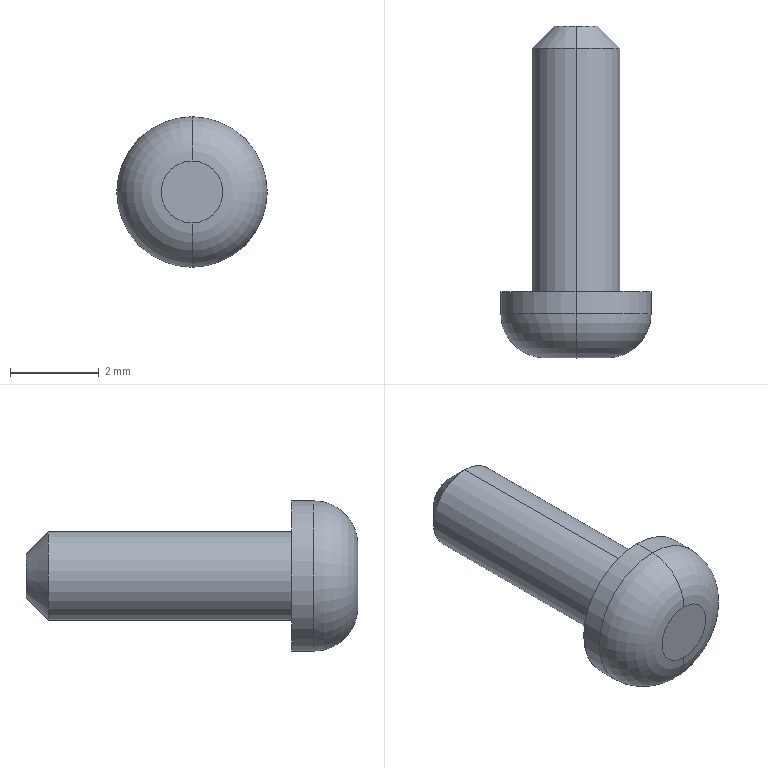Part | SolidWorks | features Chamfer 1, Extrusion 1, Fillet 1, ICE 1 | 1 solid | 11 faces | box 3.4 x 7.5 x 3.4 mm | volume 29.823 mm3 | cylinder 4 | plane 3 | torus 2 | cone 2 | commonest cylinder face diameters 2 x2 3.4 x2
STEP:
#1=CARTESIAN_POINT('',(0.,-0.5,1.7));
#2=VERTEX_POINT('',#1);
#3=CARTESIAN_POINT('',(0.,-0.5,-1.7));
#4=VERTEX_POINT('',#3);
#5=CARTESIAN_POINT('',(0.,-0.5,0.));
#6=DIRECTION('',(0.,1.,0.));
#7=DIRECTION('',(0.,0.,-1.));
#8=AXIS2_PLACEMENT_3D('',#5,#6,#7);
#9=CIRCLE('',#8,1.7);
#10=EDGE_CURVE('',#2,#4,#9,.T.);
#11=ORIENTED_EDGE('',*,*,#10,.F.);
#12=CARTESIAN_POINT('',(0.,-1.5,0.7));
#13=VERTEX_POINT('',#12);
#14=CARTESIAN_POINT('',(0.,-0.5,0.7));
#15=DIRECTION('',(1.,0.,0.));
#16=DIRECTION('',(0.,0.,-1.));
#17=AXIS2_PLACEMENT_3D('',#14,#15,#16);
#18=CIRCLE('',#17,1.);
#19=EDGE_CURVE('',#2,#13,#18,.T.);
#20=ORIENTED_EDGE('',*,*,#19,.T.);
#21=CARTESIAN_POINT('',(0.,-1.5,-0.7));
#22=VERTEX_POINT('',#21);
#23=CARTESIAN_POINT('',(0.,-1.5,0.));
#24=DIRECTION('',(0.,-1.,0.));
#25=DIRECTION('',(0.,0.,-1.));
#26=AXIS2_PLACEMENT_3D('',#23,#24,#25);
#27=CIRCLE('',#26,0.7);
#28=EDGE_CURVE('',#22,#13,#27,.T.);
#29=ORIENTED_EDGE('',*,*,#28,.F.);
#30=CARTESIAN_POINT('',(0.,-0.5,-0.7));
#31=DIRECTION('',(-1.,0.,0.));
#32=DIRECTION('',(0.,0.,1.));
#33=AXIS2_PLACEMENT_3D('',#30,#31,#32);
#34=CIRCLE('',#33,1.);
#35=EDGE_CURVE('',#4,#22,#34,.T.);
#36=ORIENTED_EDGE('',*,*,#35,.F.);
#37=EDGE_LOOP('',(#11,#20,#29,#36));
#38=FACE_OUTER_BOUND('',#37,.T.);
#39=CARTESIAN_POINT('',(0.,-0.5,0.));
#40=DIRECTION('',(0.,-1.,0.));
#41=DIRECTION('',(0.,0.,-1.));
#42=AXIS2_PLACEMENT_3D('',#39,#40,#41);
#43=TOROIDAL_SURFACE('',#42,0.7,1.);
#44=ADVANCED_FACE('',(#38),#43,.T.);
#45=ORIENTED_EDGE('',*,*,#10,.T.);
#46=CARTESIAN_POINT('',(0.,0.,-1.7));
#47=VERTEX_POINT('',#46);
#48=CARTESIAN_POINT('',(0.,-1.5,-1.7));
#49=DIRECTION('',(0.,1.,0.));
#50=VECTOR('',#49,1000.);
#51=LINE('',#48,#50);
#52=EDGE_CURVE('',#4,#47,#51,.T.);
#53=ORIENTED_EDGE('',*,*,#52,.T.);
#54=CARTESIAN_POINT('',(0.,0.,1.7));
#55=VERTEX_POINT('',#54);
#56=CARTESIAN_POINT('',(0.,0.,0.));
#57=DIRECTION('',(0.,-1.,0.));
#58=DIRECTION('',(0.,0.,-1.));
#59=AXIS2_PLACEMENT_3D('',#56,#57,#58);
#60=CIRCLE('',#59,1.7);
#61=EDGE_CURVE('',#47,#55,#60,.T.);
#62=ORIENTED_EDGE('',*,*,#61,.T.);
#63=CARTESIAN_POINT('',(0.,-1.5,1.7));
#64=DIRECTION('',(0.,1.,0.));
#65=VECTOR('',#64,1000.);
#66=LINE('',#63,#65);
#67=EDGE_CURVE('',#2,#55,#66,.T.);
#68=ORIENTED_EDGE('',*,*,#67,.F.);
#69=EDGE_LOOP('',(#45,#53,#62,#68));
#70=FACE_OUTER_BOUND('',#69,.T.);
#71=CARTESIAN_POINT('',(0.,-1.5,0.));
#72=DIRECTION('',(0.,1.,0.));
#73=DIRECTION('',(0.,0.,1.));
#74=AXIS2_PLACEMENT_3D('',#71,#72,#73);
#75=CYLINDRICAL_SURFACE('',#74,1.7);
#76=ADVANCED_FACE('',(#70),#75,.T.);
#77=CARTESIAN_POINT('',(0.,6.,0.5));
#78=VERTEX_POINT('',#77);
#79=CARTESIAN_POINT('',(0.,6.,-0.5));
#80=VERTEX_POINT('',#79);
#81=CARTESIAN_POINT('',(0.,6.,0.));
#82=DIRECTION('',(0.,1.,0.));
#83=DIRECTION('',(0.,0.,1.));
#84=AXIS2_PLACEMENT_3D('',#81,#82,#83);
#85=CIRCLE('',#84,0.5);
#86=EDGE_CURVE('',#78,#80,#85,.T.);
#87=ORIENTED_EDGE('',*,*,#86,.F.);
#88=CARTESIAN_POINT('',(0.,5.5,1.));
#89=VERTEX_POINT('',#88);
#90=CARTESIAN_POINT('',(0.,6.,0.5));
#91=DIRECTION('',(0.,-0.7071,0.7071));
#92=VECTOR('',#91,1000.);
#93=LINE('',#90,#92);
#94=EDGE_CURVE('',#78,#89,#93,.T.);
#95=ORIENTED_EDGE('',*,*,#94,.T.);
#96=CARTESIAN_POINT('',(0.,5.5,-1.));
#97=VERTEX_POINT('',#96);
#98=CARTESIAN_POINT('',(0.,5.5,0.));
#99=DIRECTION('',(0.,-1.,0.));
#100=DIRECTION('',(0.,0.,1.));
#101=AXIS2_PLACEMENT_3D('',#98,#99,#100);
#102=CIRCLE('',#101,1.);
#103=EDGE_CURVE('',#97,#89,#102,.T.);
#104=ORIENTED_EDGE('',*,*,#103,.F.);
#105=CARTESIAN_POINT('',(0.,6.,-0.5));
#106=DIRECTION('',(0.,-0.7071,-0.7071));
#107=VECTOR('',#106,1000.);
#108=LINE('',#105,#107);
#109=EDGE_CURVE('',#80,#97,#108,.T.);
#110=ORIENTED_EDGE('',*,*,#109,.F.);
#111=EDGE_LOOP('',(#87,#95,#104,#110));
#112=FACE_OUTER_BOUND('',#111,.T.);
#113=CARTESIAN_POINT('',(0.,6.,0.));
#114=DIRECTION('',(0.,-1.,0.));
#115=DIRECTION('',(0.,0.,-1.));
#116=AXIS2_PLACEMENT_3D('',#113,#114,#115);
#117=CONICAL_SURFACE('',#116,0.5,0.7854);
#118=ADVANCED_FACE('',(#112),#117,.T.);
#119=ORIENTED_EDGE('',*,*,#103,.T.);
#120=CARTESIAN_POINT('',(0.,0.,1.));
#121=VERTEX_POINT('',#120);
#122=CARTESIAN_POINT('',(0.,6.,1.));
#123=DIRECTION('',(0.,-1.,0.));
#124=VECTOR('',#123,1000.);
#125=LINE('',#122,#124);
#126=EDGE_CURVE('',#89,#121,#125,.T.);
#127=ORIENTED_EDGE('',*,*,#126,.T.);
#128=CARTESIAN_POINT('',(0.,0.,-1.));
#129=VERTEX_POINT('',#128);
#130=CARTESIAN_POINT('',(0.,0.,0.));
#131=DIRECTION('',(0.,1.,0.));
#132=DIRECTION('',(0.,0.,1.));
#133=AXIS2_PLACEMENT_3D('',#130,#131,#132);
#134=CIRCLE('',#133,1.);
#135=EDGE_CURVE('',#121,#129,#134,.T.);
#136=ORIENTED_EDGE('',*,*,#135,.T.);
#137=CARTESIAN_POINT('',(0.,6.,-1.));
#138=DIRECTION('',(0.,-1.,0.));
#139=VECTOR('',#138,1000.);
#140=LINE('',#137,#139);
#141=EDGE_CURVE('',#97,#129,#140,.T.);
#142=ORIENTED_EDGE('',*,*,#141,.F.);
#143=EDGE_LOOP('',(#119,#127,#136,#142));
#144=FACE_OUTER_BOUND('',#143,.T.);
#145=CARTESIAN_POINT('',(0.,6.,0.));
#146=DIRECTION('',(0.,-1.,0.));
#147=DIRECTION('',(0.,0.,-1.));
#148=AXIS2_PLACEMENT_3D('',#145,#146,#147);
#149=CYLINDRICAL_SURFACE('',#148,1.);
#150=ADVANCED_FACE('',(#144),#149,.T.);
#151=ORIENTED_EDGE('',*,*,#126,.F.);
#152=CARTESIAN_POINT('',(0.,5.5,0.));
#153=DIRECTION('',(0.,-1.,0.));
#154=DIRECTION('',(0.,0.,1.));
#155=AXIS2_PLACEMENT_3D('',#152,#153,#154);
#156=CIRCLE('',#155,1.);
#157=EDGE_CURVE('',#89,#97,#156,.T.);
#158=ORIENTED_EDGE('',*,*,#157,.T.);
#159=ORIENTED_EDGE('',*,*,#141,.T.);
#160=CARTESIAN_POINT('',(0.,0.,0.));
#161=DIRECTION('',(0.,1.,0.));
#162=DIRECTION('',(0.,0.,1.));
#163=AXIS2_PLACEMENT_3D('',#160,#161,#162);
#164=CIRCLE('',#163,1.);
#165=EDGE_CURVE('',#129,#121,#164,.T.);
#166=ORIENTED_EDGE('',*,*,#165,.T.);
#167=EDGE_LOOP('',(#151,#158,#159,#166));
#168=FACE_OUTER_BOUND('',#167,.T.);
#169=CARTESIAN_POINT('',(0.,6.,0.));
#170=DIRECTION('',(0.,-1.,0.));
#171=DIRECTION('',(0.,0.,-1.));
#172=AXIS2_PLACEMENT_3D('',#169,#170,#171);
#173=CYLINDRICAL_SURFACE('',#172,1.);
#174=ADVANCED_FACE('',(#168),#173,.T.);
#175=CARTESIAN_POINT('',(0.,6.,0.));
#176=DIRECTION('',(0.,1.,0.));
#177=DIRECTION('',(0.,0.,1.));
#178=AXIS2_PLACEMENT_3D('',#175,#176,#177);
#179=CIRCLE('',#178,0.5);
#180=EDGE_CURVE('',#80,#78,#179,.T.);
#181=ORIENTED_EDGE('',*,*,#180,.T.);
#182=ORIENTED_EDGE('',*,*,#86,.T.);
#183=EDGE_LOOP('',(#181,#182));
#184=FACE_OUTER_BOUND('',#183,.T.);
#185=CARTESIAN_POINT('',(0.,6.,0.));
#186=DIRECTION('',(0.,1.,0.));
#187=DIRECTION('',(0.,0.,1.));
#188=AXIS2_PLACEMENT_3D('',#185,#186,#187);
#189=PLANE('',#188);
#190=ADVANCED_FACE('',(#184),#189,.T.);
#191=ORIENTED_EDGE('',*,*,#94,.F.);
#192=ORIENTED_EDGE('',*,*,#180,.F.);
#193=ORIENTED_EDGE('',*,*,#109,.T.);
#194=ORIENTED_EDGE('',*,*,#157,.F.);
#195=EDGE_LOOP('',(#191,#192,#193,#194));
#196=FACE_OUTER_BOUND('',#195,.T.);
#197=CARTESIAN_POINT('',(0.,6.,0.));
#198=DIRECTION('',(0.,-1.,0.));
#199=DIRECTION('',(0.,0.,-1.));
#200=AXIS2_PLACEMENT_3D('',#197,#198,#199);
#201=CONICAL_SURFACE('',#200,0.5,0.7854);
#202=ADVANCED_FACE('',(#196),#201,.T.);
#203=ORIENTED_EDGE('',*,*,#52,.F.);
#204=CARTESIAN_POINT('',(0.,-0.5,0.));
#205=DIRECTION('',(0.,1.,0.));
#206=DIRECTION('',(0.,0.,-1.));
#207=AXIS2_PLACEMENT_3D('',#204,#205,#206);
#208=CIRCLE('',#207,1.7);
#209=EDGE_CURVE('',#4,#2,#208,.T.);
#210=ORIENTED_EDGE('',*,*,#209,.T.);
#211=ORIENTED_EDGE('',*,*,#67,.T.);
#212=CARTESIAN_POINT('',(0.,0.,0.));
#213=DIRECTION('',(0.,-1.,0.));
#214=DIRECTION('',(0.,0.,-1.));
#215=AXIS2_PLACEMENT_3D('',#212,#213,#214);
#216=CIRCLE('',#215,1.7);
#217=EDGE_CURVE('',#55,#47,#216,.T.);
#218=ORIENTED_EDGE('',*,*,#217,.T.);
#219=EDGE_LOOP('',(#203,#210,#211,#218));
#220=FACE_OUTER_BOUND('',#219,.T.);
#221=CARTESIAN_POINT('',(0.,-1.5,0.));
#222=DIRECTION('',(0.,1.,0.));
#223=DIRECTION('',(0.,0.,1.));
#224=AXIS2_PLACEMENT_3D('',#221,#222,#223);
#225=CYLINDRICAL_SURFACE('',#224,1.7);
#226=ADVANCED_FACE('',(#220),#225,.T.);
#227=ORIENTED_EDGE('',*,*,#28,.T.);
#228=CARTESIAN_POINT('',(0.,-1.5,0.));
#229=DIRECTION('',(0.,-1.,0.));
#230=DIRECTION('',(0.,0.,-1.));
#231=AXIS2_PLACEMENT_3D('',#228,#229,#230);
#232=CIRCLE('',#231,0.7);
#233=EDGE_CURVE('',#13,#22,#232,.T.);
#234=ORIENTED_EDGE('',*,*,#233,.T.);
#235=EDGE_LOOP('',(#227,#234));
#236=FACE_OUTER_BOUND('',#235,.T.);
#237=CARTESIAN_POINT('',(0.,-1.5,0.));
#238=DIRECTION('',(0.,-1.,0.));
#239=DIRECTION('',(0.,0.,-1.));
#240=AXIS2_PLACEMENT_3D('',#237,#238,#239);
#241=PLANE('',#240);
#242=ADVANCED_FACE('',(#236),#241,.T.);
#243=ORIENTED_EDGE('',*,*,#165,.F.);
#244=ORIENTED_EDGE('',*,*,#135,.F.);
#245=EDGE_LOOP('',(#243,#244));
#246=FACE_BOUND('',#245,.T.);
#247=ORIENTED_EDGE('',*,*,#217,.F.);
#248=ORIENTED_EDGE('',*,*,#61,.F.);
#249=EDGE_LOOP('',(#247,#248));
#250=FACE_OUTER_BOUND('',#249,.T.);
#251=CARTESIAN_POINT('',(0.,0.,0.));
#252=DIRECTION('',(0.,-1.,0.));
#253=DIRECTION('',(0.,0.,-1.));
#254=AXIS2_PLACEMENT_3D('',#251,#252,#253);
#255=PLANE('',#254);
#256=ADVANCED_FACE('',(#246,#250),#255,.F.);
#257=ORIENTED_EDGE('',*,*,#19,.F.);
#258=ORIENTED_EDGE('',*,*,#209,.F.);
#259=ORIENTED_EDGE('',*,*,#35,.T.);
#260=ORIENTED_EDGE('',*,*,#233,.F.);
#261=EDGE_LOOP('',(#257,#258,#259,#260));
#262=FACE_OUTER_BOUND('',#261,.T.);
#263=CARTESIAN_POINT('',(0.,-0.5,0.));
#264=DIRECTION('',(0.,-1.,0.));
#265=DIRECTION('',(0.,0.,-1.));
#266=AXIS2_PLACEMENT_3D('',#263,#264,#265);
#267=TOROIDAL_SURFACE('',#266,0.7,1.);
#268=ADVANCED_FACE('',(#262),#267,.T.);
#269=CLOSED_SHELL('',(#44,#76,#118,#150,#174,#190,#202,#226,#242,#256,#268));
#270=MANIFOLD_SOLID_BREP('',#269);
#271=CARTESIAN_POINT('',(0.,0.,0.));
#272=DIRECTION('',(0.,0.,1.));
#273=DIRECTION('',(1.,0.,0.));
#274=AXIS2_PLACEMENT_3D('',#271,#272,#273);
#275=(LENGTH_UNIT()NAMED_UNIT(*)SI_UNIT(.MILLI.,.METRE.));
#276=UNCERTAINTY_MEASURE_WITH_UNIT(LENGTH_MEASURE(0.00001),#275,'','');
#277=(NAMED_UNIT(*)PLANE_ANGLE_UNIT()SI_UNIT($,.RADIAN.));
#278=(NAMED_UNIT(*)SI_UNIT($,.STERADIAN.)SOLID_ANGLE_UNIT());
#279=(GEOMETRIC_REPRESENTATION_CONTEXT(3)GLOBAL_UNCERTAINTY_ASSIGNED_CONTEXT((#276))GLOBAL_UNIT_ASSIGNED_CONTEXT((#275,#277,#278))REPRESENTATION_CONTEXT('',''));
#280=ADVANCED_BREP_SHAPE_REPRESENTATION('',(#270,#274),#279);